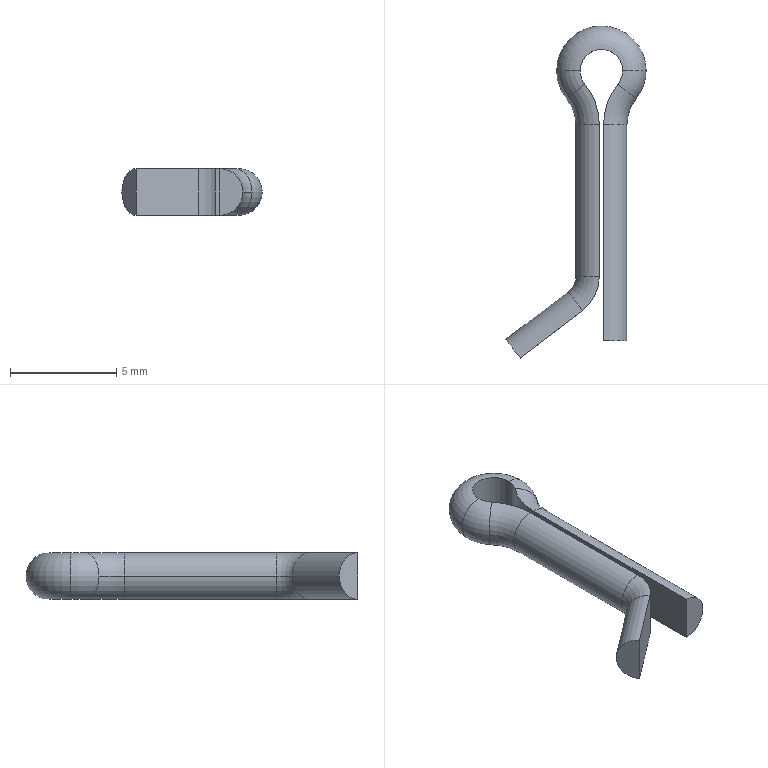Part | NX | features BREP 1 | 1 solid | 25 faces | box 6.586 x 15.587 x 2.2 mm | volume 61.721 mm3 | cylinder 11 | torus 9 | plane 5 | commonest cylinder face diameters 2.2 x5 2 x3 6 x2 4 x1
STEP:
#1=CARTESIAN_POINT('',(1.2,-6.604,4.));
#2=VERTEX_POINT('',#1);
#3=CARTESIAN_POINT('',(1.2,3.554,4.));
#4=VERTEX_POINT('',#3);
#5=CARTESIAN_POINT('',(1.2,-6.604,4.));
#6=DIRECTION('',(0.,1.,0.));
#7=VECTOR('',#6,1000.);
#8=LINE('',#5,#7);
#9=EDGE_CURVE('',#2,#4,#8,.T.);
#10=ORIENTED_EDGE('',*,*,#9,.F.);
#11=CARTESIAN_POINT('',(0.1,-6.604,2.9));
#12=VERTEX_POINT('',#11);
#13=CARTESIAN_POINT('',(0.1,-6.604,4.));
#14=DIRECTION('',(0.,-1.,0.));
#15=DIRECTION('',(0.,0.,-1.));
#16=AXIS2_PLACEMENT_3D('',#13,#14,#15);
#17=CIRCLE('',#16,1.1);
#18=EDGE_CURVE('',#12,#2,#17,.T.);
#19=ORIENTED_EDGE('',*,*,#18,.F.);
#20=CARTESIAN_POINT('',(0.1,3.554,2.9));
#21=VERTEX_POINT('',#20);
#22=CARTESIAN_POINT('',(0.1,-6.604,2.9));
#23=DIRECTION('',(0.,1.,0.));
#24=VECTOR('',#23,1000.);
#25=LINE('',#22,#24);
#26=EDGE_CURVE('',#12,#21,#25,.T.);
#27=ORIENTED_EDGE('',*,*,#26,.T.);
#28=CARTESIAN_POINT('',(0.1,3.554,4.));
#29=DIRECTION('',(0.,1.,0.));
#30=DIRECTION('',(1.,0.,0.));
#31=AXIS2_PLACEMENT_3D('',#28,#29,#30);
#32=CIRCLE('',#31,1.1);
#33=EDGE_CURVE('',#4,#21,#32,.T.);
#34=ORIENTED_EDGE('',*,*,#33,.F.);
#35=EDGE_LOOP('',(#10,#19,#27,#34));
#36=FACE_BOUND('',#35,.T.);
#37=CARTESIAN_POINT('',(0.1,3.554,4.));
#38=DIRECTION('',(0.,-1.,0.));
#39=DIRECTION('',(-1.,0.,0.));
#40=AXIS2_PLACEMENT_3D('',#37,#38,#39);
#41=CYLINDRICAL_SURFACE('',#40,1.1);
#42=ADVANCED_FACE('',(#36),#41,.T.);
#43=CARTESIAN_POINT('',(1.627,4.754,4.));
#44=VERTEX_POINT('',#43);
#45=CARTESIAN_POINT('',(3.1,3.554,4.));
#46=DIRECTION('',(0.,0.,-1.));
#47=DIRECTION('',(-1.,0.,0.));
#48=AXIS2_PLACEMENT_3D('',#45,#46,#47);
#49=CIRCLE('',#48,1.9);
#50=EDGE_CURVE('',#4,#44,#49,.T.);
#51=ORIENTED_EDGE('',*,*,#50,.F.);
#52=ORIENTED_EDGE('',*,*,#33,.T.);
#53=CARTESIAN_POINT('',(0.775,5.449,2.9));
#54=VERTEX_POINT('',#53);
#55=CARTESIAN_POINT('',(3.1,3.554,2.9));
#56=DIRECTION('',(0.,0.,-1.));
#57=DIRECTION('',(-1.,0.,0.));
#58=AXIS2_PLACEMENT_3D('',#55,#56,#57);
#59=CIRCLE('',#58,3.);
#60=EDGE_CURVE('',#21,#54,#59,.T.);
#61=ORIENTED_EDGE('',*,*,#60,.T.);
#62=CARTESIAN_POINT('',(0.775,5.449,4.));
#63=DIRECTION('',(-0.632,-0.775,0.));
#64=DIRECTION('',(0.,0.,-1.));
#65=AXIS2_PLACEMENT_3D('',#62,#63,#64);
#66=CIRCLE('',#65,1.1);
#67=EDGE_CURVE('',#54,#44,#66,.T.);
#68=ORIENTED_EDGE('',*,*,#67,.T.);
#69=EDGE_LOOP('',(#51,#52,#61,#68));
#70=FACE_BOUND('',#69,.T.);
#71=CARTESIAN_POINT('',(3.1,3.554,4.));
#72=DIRECTION('',(0.,0.,1.));
#73=DIRECTION('',(-1.,0.,0.));
#74=AXIS2_PLACEMENT_3D('',#71,#72,#73);
#75=TOROIDAL_SURFACE('',#74,3.,1.1);
#76=ADVANCED_FACE('',(#70),#75,.T.);
#77=CARTESIAN_POINT('',(2.1,6.081,4.));
#78=VERTEX_POINT('',#77);
#79=CARTESIAN_POINT('',(1.,6.081,5.1));
#80=VERTEX_POINT('',#79);
#81=CARTESIAN_POINT('',(1.,6.081,4.));
#82=DIRECTION('',(0.,-1.,0.));
#83=DIRECTION('',(1.,0.,0.));
#84=AXIS2_PLACEMENT_3D('',#81,#82,#83);
#85=CIRCLE('',#84,1.1);
#86=EDGE_CURVE('',#78,#80,#85,.T.);
#87=ORIENTED_EDGE('',*,*,#86,.T.);
#88=CARTESIAN_POINT('',(0.775,5.449,5.1));
#89=VERTEX_POINT('',#88);
#90=CARTESIAN_POINT('',(0.,6.081,5.1));
#91=DIRECTION('',(0.,0.,-1.));
#92=DIRECTION('',(1.,0.,0.));
#93=AXIS2_PLACEMENT_3D('',#90,#91,#92);
#94=CIRCLE('',#93,1.);
#95=EDGE_CURVE('',#80,#89,#94,.T.);
#96=ORIENTED_EDGE('',*,*,#95,.T.);
#97=CARTESIAN_POINT('',(0.775,5.449,4.));
#98=DIRECTION('',(-0.632,-0.775,0.));
#99=DIRECTION('',(0.775,-0.632,0.));
#100=AXIS2_PLACEMENT_3D('',#97,#98,#99);
#101=CIRCLE('',#100,1.1);
#102=EDGE_CURVE('',#44,#89,#101,.T.);
#103=ORIENTED_EDGE('',*,*,#102,.F.);
#104=ORIENTED_EDGE('',*,*,#67,.F.);
#105=CARTESIAN_POINT('',(1.,6.081,2.9));
#106=VERTEX_POINT('',#105);
#107=CARTESIAN_POINT('',(0.,6.081,2.9));
#108=DIRECTION('',(0.,0.,1.));
#109=DIRECTION('',(0.775,-0.632,0.));
#110=AXIS2_PLACEMENT_3D('',#107,#108,#109);
#111=CIRCLE('',#110,1.);
#112=EDGE_CURVE('',#54,#106,#111,.T.);
#113=ORIENTED_EDGE('',*,*,#112,.T.);
#114=CARTESIAN_POINT('',(1.,6.081,4.));
#115=DIRECTION('',(0.,-1.,0.));
#116=DIRECTION('',(0.,0.,-1.));
#117=AXIS2_PLACEMENT_3D('',#114,#115,#116);
#118=CIRCLE('',#117,1.1);
#119=EDGE_CURVE('',#106,#78,#118,.T.);
#120=ORIENTED_EDGE('',*,*,#119,.T.);
#121=EDGE_LOOP('',(#87,#96,#103,#104,#113,#120));
#122=FACE_BOUND('',#121,.T.);
#123=CARTESIAN_POINT('',(0.,6.081,4.));
#124=DIRECTION('',(0.,0.,-1.));
#125=DIRECTION('',(-1.,0.,0.));
#126=AXIS2_PLACEMENT_3D('',#123,#124,#125);
#127=DEGENERATE_TOROIDAL_SURFACE('',#126,1.,1.1,.T.);
#128=ADVANCED_FACE('',(#122),#127,.T.);
#129=ORIENTED_EDGE('',*,*,#86,.F.);
#130=ORIENTED_EDGE('',*,*,#119,.F.);
#131=CARTESIAN_POINT('',(-1.,6.081,2.9));
#132=VERTEX_POINT('',#131);
#133=CARTESIAN_POINT('',(0.,6.081,2.9));
#134=DIRECTION('',(0.,0.,1.));
#135=DIRECTION('',(1.,0.,0.));
#136=AXIS2_PLACEMENT_3D('',#133,#134,#135);
#137=CIRCLE('',#136,1.);
#138=EDGE_CURVE('',#106,#132,#137,.T.);
#139=ORIENTED_EDGE('',*,*,#138,.T.);
#140=CARTESIAN_POINT('',(-2.1,6.081,4.));
#141=VERTEX_POINT('',#140);
#142=CARTESIAN_POINT('',(-1.,6.081,4.));
#143=DIRECTION('',(0.,1.,0.));
#144=DIRECTION('',(0.,0.,-1.));
#145=AXIS2_PLACEMENT_3D('',#142,#143,#144);
#146=CIRCLE('',#145,1.1);
#147=EDGE_CURVE('',#132,#141,#146,.T.);
#148=ORIENTED_EDGE('',*,*,#147,.T.);
#149=CARTESIAN_POINT('',(-1.,6.081,5.1));
#150=VERTEX_POINT('',#149);
#151=CARTESIAN_POINT('',(-1.,6.081,4.));
#152=DIRECTION('',(0.,1.,0.));
#153=DIRECTION('',(-1.,0.,0.));
#154=AXIS2_PLACEMENT_3D('',#151,#152,#153);
#155=CIRCLE('',#154,1.1);
#156=EDGE_CURVE('',#141,#150,#155,.T.);
#157=ORIENTED_EDGE('',*,*,#156,.T.);
#158=CARTESIAN_POINT('',(0.,6.081,5.1));
#159=DIRECTION('',(0.,0.,-1.));
#160=DIRECTION('',(-1.,0.,0.));
#161=AXIS2_PLACEMENT_3D('',#158,#159,#160);
#162=CIRCLE('',#161,1.);
#163=EDGE_CURVE('',#150,#80,#162,.T.);
#164=ORIENTED_EDGE('',*,*,#163,.T.);
#165=EDGE_LOOP('',(#129,#130,#139,#148,#157,#164));
#166=FACE_BOUND('',#165,.T.);
#167=CARTESIAN_POINT('',(0.,6.081,4.));
#168=DIRECTION('',(0.,0.,-1.));
#169=DIRECTION('',(-1.,0.,0.));
#170=AXIS2_PLACEMENT_3D('',#167,#168,#169);
#171=DEGENERATE_TOROIDAL_SURFACE('',#170,1.,1.1,.T.);
#172=ADVANCED_FACE('',(#166),#171,.T.);
#173=ORIENTED_EDGE('',*,*,#163,.F.);
#174=CARTESIAN_POINT('',(-1.,6.081,2.9));
#175=DIRECTION('',(0.,0.,1.));
#176=VECTOR('',#175,1000.);
#177=LINE('',#174,#176);
#178=EDGE_CURVE('',#132,#150,#177,.T.);
#179=ORIENTED_EDGE('',*,*,#178,.F.);
#180=ORIENTED_EDGE('',*,*,#138,.F.);
#181=CARTESIAN_POINT('',(1.,6.081,2.9));
#182=DIRECTION('',(0.,0.,1.));
#183=VECTOR('',#182,1000.);
#184=LINE('',#181,#183);
#185=EDGE_CURVE('',#106,#80,#184,.T.);
#186=ORIENTED_EDGE('',*,*,#185,.T.);
#187=EDGE_LOOP('',(#173,#179,#180,#186));
#188=FACE_BOUND('',#187,.T.);
#189=CARTESIAN_POINT('',(0.,6.081,4.));
#190=DIRECTION('',(0.,0.,-1.));
#191=DIRECTION('',(1.,0.,0.));
#192=AXIS2_PLACEMENT_3D('',#189,#190,#191);
#193=CYLINDRICAL_SURFACE('',#192,1.);
#194=ADVANCED_FACE('',(#188),#193,.F.);
#195=ORIENTED_EDGE('',*,*,#185,.F.);
#196=ORIENTED_EDGE('',*,*,#112,.F.);
#197=CARTESIAN_POINT('',(0.775,5.449,5.1));
#198=DIRECTION('',(0.,0.,-1.));
#199=VECTOR('',#198,1000.);
#200=LINE('',#197,#199);
#201=EDGE_CURVE('',#89,#54,#200,.T.);
#202=ORIENTED_EDGE('',*,*,#201,.F.);
#203=ORIENTED_EDGE('',*,*,#95,.F.);
#204=EDGE_LOOP('',(#195,#196,#202,#203));
#205=FACE_BOUND('',#204,.T.);
#206=CARTESIAN_POINT('',(0.,6.081,4.));
#207=DIRECTION('',(0.,0.,-1.));
#208=DIRECTION('',(1.,0.,0.));
#209=AXIS2_PLACEMENT_3D('',#206,#207,#208);
#210=CYLINDRICAL_SURFACE('',#209,1.);
#211=ADVANCED_FACE('',(#205),#210,.F.);
#212=ORIENTED_EDGE('',*,*,#60,.F.);
#213=CARTESIAN_POINT('',(0.1,3.554,5.1));
#214=VERTEX_POINT('',#213);
#215=CARTESIAN_POINT('',(0.1,3.554,2.9));
#216=DIRECTION('',(0.,0.,1.));
#217=VECTOR('',#216,1000.);
#218=LINE('',#215,#217);
#219=EDGE_CURVE('',#21,#214,#218,.T.);
#220=ORIENTED_EDGE('',*,*,#219,.T.);
#221=CARTESIAN_POINT('',(3.1,3.554,5.1));
#222=DIRECTION('',(0.,0.,1.));
#223=DIRECTION('',(-0.775,0.632,0.));
#224=AXIS2_PLACEMENT_3D('',#221,#222,#223);
#225=CIRCLE('',#224,3.);
#226=EDGE_CURVE('',#89,#214,#225,.T.);
#227=ORIENTED_EDGE('',*,*,#226,.F.);
#228=ORIENTED_EDGE('',*,*,#201,.T.);
#229=EDGE_LOOP('',(#212,#220,#227,#228));
#230=FACE_BOUND('',#229,.T.);
#231=CARTESIAN_POINT('',(3.1,3.554,4.));
#232=DIRECTION('',(0.,0.,1.));
#233=DIRECTION('',(-1.,0.,0.));
#234=AXIS2_PLACEMENT_3D('',#231,#232,#233);
#235=CYLINDRICAL_SURFACE('',#234,3.);
#236=ADVANCED_FACE('',(#230),#235,.T.);
#237=ORIENTED_EDGE('',*,*,#102,.T.);
#238=ORIENTED_EDGE('',*,*,#226,.T.);
#239=CARTESIAN_POINT('',(0.1,3.554,4.));
#240=DIRECTION('',(0.,1.,0.));
#241=DIRECTION('',(0.,0.,1.));
#242=AXIS2_PLACEMENT_3D('',#239,#240,#241);
#243=CIRCLE('',#242,1.1);
#244=EDGE_CURVE('',#214,#4,#243,.T.);
#245=ORIENTED_EDGE('',*,*,#244,.T.);
#246=ORIENTED_EDGE('',*,*,#50,.T.);
#247=EDGE_LOOP('',(#237,#238,#245,#246));
#248=FACE_BOUND('',#247,.T.);
#249=CARTESIAN_POINT('',(3.1,3.554,4.));
#250=DIRECTION('',(0.,0.,1.));
#251=DIRECTION('',(-1.,0.,0.));
#252=AXIS2_PLACEMENT_3D('',#249,#250,#251);
#253=TOROIDAL_SURFACE('',#252,3.,1.1);
#254=ADVANCED_FACE('',(#248),#253,.T.);
#255=ORIENTED_EDGE('',*,*,#244,.F.);
#256=CARTESIAN_POINT('',(0.1,-6.604,5.1));
#257=VERTEX_POINT('',#256);
#258=CARTESIAN_POINT('',(0.1,3.554,5.1));
#259=DIRECTION('',(0.,-1.,0.));
#260=VECTOR('',#259,1000.);
#261=LINE('',#258,#260);
#262=EDGE_CURVE('',#214,#257,#261,.T.);
#263=ORIENTED_EDGE('',*,*,#262,.T.);
#264=CARTESIAN_POINT('',(0.1,-6.604,4.));
#265=DIRECTION('',(0.,-1.,0.));
#266=DIRECTION('',(1.,0.,0.));
#267=AXIS2_PLACEMENT_3D('',#264,#265,#266);
#268=CIRCLE('',#267,1.1);
#269=EDGE_CURVE('',#2,#257,#268,.T.);
#270=ORIENTED_EDGE('',*,*,#269,.F.);
#271=ORIENTED_EDGE('',*,*,#9,.T.);
#272=EDGE_LOOP('',(#255,#263,#270,#271));
#273=FACE_BOUND('',#272,.T.);
#274=CARTESIAN_POINT('',(0.1,3.554,4.));
#275=DIRECTION('',(0.,-1.,0.));
#276=DIRECTION('',(-1.,0.,0.));
#277=AXIS2_PLACEMENT_3D('',#274,#275,#276);
#278=CYLINDRICAL_SURFACE('',#277,1.1);
#279=ADVANCED_FACE('',(#273),#278,.T.);
#280=CARTESIAN_POINT('',(0.1,-6.604,5.1));
#281=DIRECTION('',(0.,0.,-1.));
#282=VECTOR('',#281,1000.);
#283=LINE('',#280,#282);
#284=EDGE_CURVE('',#257,#12,#283,.T.);
#285=ORIENTED_EDGE('',*,*,#284,.T.);
#286=ORIENTED_EDGE('',*,*,#18,.T.);
#287=ORIENTED_EDGE('',*,*,#269,.T.);
#288=EDGE_LOOP('',(#285,#286,#287));
#289=FACE_BOUND('',#288,.T.);
#290=CARTESIAN_POINT('',(0.1,-6.604,4.));
#291=DIRECTION('',(0.,1.,0.));
#292=DIRECTION('',(1.,0.,0.));
#293=AXIS2_PLACEMENT_3D('',#290,#291,#292);
#294=PLANE('',#293);
#295=ADVANCED_FACE('',(#289),#294,.F.);
#296=ORIENTED_EDGE('',*,*,#26,.F.);
#297=ORIENTED_EDGE('',*,*,#284,.F.);
#298=ORIENTED_EDGE('',*,*,#262,.F.);
#299=ORIENTED_EDGE('',*,*,#219,.F.);
#300=EDGE_LOOP('',(#296,#297,#298,#299));
#301=FACE_BOUND('',#300,.T.);
#302=CARTESIAN_POINT('',(0.1,3.554,5.1));
#303=DIRECTION('',(1.,0.,0.));
#304=DIRECTION('',(0.,-1.,0.));
#305=AXIS2_PLACEMENT_3D('',#302,#303,#304);
#306=PLANE('',#305);
#307=ADVANCED_FACE('',(#301),#306,.F.);
#308=CARTESIAN_POINT('',(-0.775,5.449,5.1));
#309=VERTEX_POINT('',#308);
#310=CARTESIAN_POINT('',(0.,6.081,5.1));
#311=DIRECTION('',(0.,0.,-1.));
#312=DIRECTION('',(-0.775,-0.632,0.));
#313=AXIS2_PLACEMENT_3D('',#310,#311,#312);
#314=CIRCLE('',#313,1.);
#315=EDGE_CURVE('',#309,#150,#314,.T.);
#316=ORIENTED_EDGE('',*,*,#315,.F.);
#317=CARTESIAN_POINT('',(-0.775,5.449,2.9));
#318=VERTEX_POINT('',#317);
#319=CARTESIAN_POINT('',(-0.775,5.449,5.1));
#320=DIRECTION('',(0.,0.,-1.));
#321=VECTOR('',#320,1000.);
#322=LINE('',#319,#321);
#323=EDGE_CURVE('',#309,#318,#322,.T.);
#324=ORIENTED_EDGE('',*,*,#323,.T.);
#325=CARTESIAN_POINT('',(0.,6.081,2.9));
#326=DIRECTION('',(0.,0.,1.));
#327=DIRECTION('',(-1.,0.,0.));
#328=AXIS2_PLACEMENT_3D('',#325,#326,#327);
#329=CIRCLE('',#328,1.);
#330=EDGE_CURVE('',#132,#318,#329,.T.);
#331=ORIENTED_EDGE('',*,*,#330,.F.);
#332=ORIENTED_EDGE('',*,*,#178,.T.);
#333=EDGE_LOOP('',(#316,#324,#331,#332));
#334=FACE_BOUND('',#333,.T.);
#335=CARTESIAN_POINT('',(0.,6.081,4.));
#336=DIRECTION('',(0.,0.,-1.));
#337=DIRECTION('',(1.,0.,0.));
#338=AXIS2_PLACEMENT_3D('',#335,#336,#337);
#339=CYLINDRICAL_SURFACE('',#338,1.);
#340=ADVANCED_FACE('',(#334),#339,.F.);
#341=ORIENTED_EDGE('',*,*,#156,.F.);
#342=ORIENTED_EDGE('',*,*,#147,.F.);
#343=ORIENTED_EDGE('',*,*,#330,.T.);
#344=CARTESIAN_POINT('',(-1.627,4.754,4.));
#345=VERTEX_POINT('',#344);
#346=CARTESIAN_POINT('',(-0.775,5.449,4.));
#347=DIRECTION('',(-0.632,0.775,0.));
#348=DIRECTION('',(0.,0.,-1.));
#349=AXIS2_PLACEMENT_3D('',#346,#347,#348);
#350=CIRCLE('',#349,1.1);
#351=EDGE_CURVE('',#318,#345,#350,.T.);
#352=ORIENTED_EDGE('',*,*,#351,.T.);
#353=CARTESIAN_POINT('',(-0.775,5.449,4.));
#354=DIRECTION('',(-0.632,0.775,0.));
#355=DIRECTION('',(-0.775,-0.632,0.));
#356=AXIS2_PLACEMENT_3D('',#353,#354,#355);
#357=CIRCLE('',#356,1.1);
#358=EDGE_CURVE('',#345,#309,#357,.T.);
#359=ORIENTED_EDGE('',*,*,#358,.T.);
#360=ORIENTED_EDGE('',*,*,#315,.T.);
#361=EDGE_LOOP('',(#341,#342,#343,#352,#359,#360));
#362=FACE_BOUND('',#361,.T.);
#363=CARTESIAN_POINT('',(0.,6.081,4.));
#364=DIRECTION('',(0.,0.,-1.));
#365=DIRECTION('',(-1.,0.,0.));
#366=AXIS2_PLACEMENT_3D('',#363,#364,#365);
#367=DEGENERATE_TOROIDAL_SURFACE('',#366,1.,1.1,.T.);
#368=ADVANCED_FACE('',(#362),#367,.T.);
#369=CARTESIAN_POINT('',(-1.2,3.554,4.));
#370=VERTEX_POINT('',#369);
#371=CARTESIAN_POINT('',(-0.1,3.554,5.1));
#372=VERTEX_POINT('',#371);
#373=CARTESIAN_POINT('',(-0.1,3.554,4.));
#374=DIRECTION('',(0.,1.,0.));
#375=DIRECTION('',(-1.,0.,0.));
#376=AXIS2_PLACEMENT_3D('',#373,#374,#375);
#377=CIRCLE('',#376,1.1);
#378=EDGE_CURVE('',#370,#372,#377,.T.);
#379=ORIENTED_EDGE('',*,*,#378,.T.);
#380=CARTESIAN_POINT('',(-3.1,3.554,5.1));
#381=DIRECTION('',(0.,0.,1.));
#382=DIRECTION('',(1.,0.,0.));
#383=AXIS2_PLACEMENT_3D('',#380,#381,#382);
#384=CIRCLE('',#383,3.);
#385=EDGE_CURVE('',#372,#309,#384,.T.);
#386=ORIENTED_EDGE('',*,*,#385,.T.);
#387=ORIENTED_EDGE('',*,*,#358,.F.);
#388=CARTESIAN_POINT('',(-3.1,3.554,4.));
#389=DIRECTION('',(0.,0.,-1.));
#390=DIRECTION('',(0.775,0.632,0.));
#391=AXIS2_PLACEMENT_3D('',#388,#389,#390);
#392=CIRCLE('',#391,1.9);
#393=EDGE_CURVE('',#345,#370,#392,.T.);
#394=ORIENTED_EDGE('',*,*,#393,.T.);
#395=EDGE_LOOP('',(#379,#386,#387,#394));
#396=FACE_BOUND('',#395,.T.);
#397=CARTESIAN_POINT('',(-3.1,3.554,4.));
#398=DIRECTION('',(0.,0.,1.));
#399=DIRECTION('',(-1.,0.,0.));
#400=AXIS2_PLACEMENT_3D('',#397,#398,#399);
#401=TOROIDAL_SURFACE('',#400,3.,1.1);
#402=ADVANCED_FACE('',(#396),#401,.T.);
#403=ORIENTED_EDGE('',*,*,#393,.F.);
#404=ORIENTED_EDGE('',*,*,#351,.F.);
#405=CARTESIAN_POINT('',(-0.1,3.554,2.9));
#406=VERTEX_POINT('',#405);
#407=CARTESIAN_POINT('',(-3.1,3.554,2.9));
#408=DIRECTION('',(0.,0.,-1.));
#409=DIRECTION('',(0.775,0.632,0.));
#410=AXIS2_PLACEMENT_3D('',#407,#408,#409);
#411=CIRCLE('',#410,3.);
#412=EDGE_CURVE('',#318,#406,#411,.T.);
#413=ORIENTED_EDGE('',*,*,#412,.T.);
#414=CARTESIAN_POINT('',(-0.1,3.554,4.));
#415=DIRECTION('',(0.,1.,0.));
#416=DIRECTION('',(0.,0.,-1.));
#417=AXIS2_PLACEMENT_3D('',#414,#415,#416);
#418=CIRCLE('',#417,1.1);
#419=EDGE_CURVE('',#406,#370,#418,.T.);
#420=ORIENTED_EDGE('',*,*,#419,.T.);
#421=EDGE_LOOP('',(#403,#404,#413,#420));
#422=FACE_BOUND('',#421,.T.);
#423=CARTESIAN_POINT('',(-3.1,3.554,4.));
#424=DIRECTION('',(0.,0.,1.));
#425=DIRECTION('',(-1.,0.,0.));
#426=AXIS2_PLACEMENT_3D('',#423,#424,#425);
#427=TOROIDAL_SURFACE('',#426,3.,1.1);
#428=ADVANCED_FACE('',(#422),#427,.T.);
#429=CARTESIAN_POINT('',(-1.2,-3.591,4.));
#430=VERTEX_POINT('',#429);
#431=CARTESIAN_POINT('',(-1.2,3.554,4.));
#432=DIRECTION('',(0.,-1.,0.));
#433=VECTOR('',#432,1000.);
#434=LINE('',#431,#433);
#435=EDGE_CURVE('',#370,#430,#434,.T.);
#436=ORIENTED_EDGE('',*,*,#435,.F.);
#437=ORIENTED_EDGE('',*,*,#419,.F.);
#438=CARTESIAN_POINT('',(-0.1,-3.591,2.9));
#439=VERTEX_POINT('',#438);
#440=CARTESIAN_POINT('',(-0.1,3.554,2.9));
#441=DIRECTION('',(0.,-1.,0.));
#442=VECTOR('',#441,1000.);
#443=LINE('',#440,#442);
#444=EDGE_CURVE('',#406,#439,#443,.T.);
#445=ORIENTED_EDGE('',*,*,#444,.T.);
#446=CARTESIAN_POINT('',(-0.1,-3.591,4.));
#447=DIRECTION('',(0.,-1.,0.));
#448=DIRECTION('',(-1.,0.,0.));
#449=AXIS2_PLACEMENT_3D('',#446,#447,#448);
#450=CIRCLE('',#449,1.1);
#451=EDGE_CURVE('',#430,#439,#450,.T.);
#452=ORIENTED_EDGE('',*,*,#451,.F.);
#453=EDGE_LOOP('',(#436,#437,#445,#452));
#454=FACE_BOUND('',#453,.T.);
#455=CARTESIAN_POINT('',(-0.1,-3.591,4.));
#456=DIRECTION('',(0.,1.,0.));
#457=DIRECTION('',(1.,0.,0.));
#458=AXIS2_PLACEMENT_3D('',#455,#456,#457);
#459=CYLINDRICAL_SURFACE('',#458,1.1);
#460=ADVANCED_FACE('',(#454),#459,.T.);
#461=CARTESIAN_POINT('',(-1.556,-4.308,4.));
#462=VERTEX_POINT('',#461);
#463=CARTESIAN_POINT('',(-2.1,-3.591,4.));
#464=DIRECTION('',(0.,0.,-1.));
#465=DIRECTION('',(1.,0.,0.));
#466=AXIS2_PLACEMENT_3D('',#463,#464,#465);
#467=CIRCLE('',#466,0.9);
#468=EDGE_CURVE('',#430,#462,#467,.T.);
#469=ORIENTED_EDGE('',*,*,#468,.F.);
#470=ORIENTED_EDGE('',*,*,#451,.T.);
#471=CARTESIAN_POINT('',(-0.8919,-5.185,2.9));
#472=VERTEX_POINT('',#471);
#473=CARTESIAN_POINT('',(-2.1,-3.591,2.9));
#474=DIRECTION('',(0.,0.,-1.));
#475=DIRECTION('',(1.,0.,0.));
#476=AXIS2_PLACEMENT_3D('',#473,#474,#475);
#477=CIRCLE('',#476,2.);
#478=EDGE_CURVE('',#439,#472,#477,.T.);
#479=ORIENTED_EDGE('',*,*,#478,.T.);
#480=CARTESIAN_POINT('',(-0.8919,-5.185,4.));
#481=DIRECTION('',(0.7969,0.6041,0.));
#482=DIRECTION('',(0.,0.,-1.));
#483=AXIS2_PLACEMENT_3D('',#480,#481,#482);
#484=CIRCLE('',#483,1.1);
#485=EDGE_CURVE('',#472,#462,#484,.T.);
#486=ORIENTED_EDGE('',*,*,#485,.T.);
#487=EDGE_LOOP('',(#469,#470,#479,#486));
#488=FACE_BOUND('',#487,.T.);
#489=CARTESIAN_POINT('',(-2.1,-3.591,4.));
#490=DIRECTION('',(0.,0.,1.));
#491=DIRECTION('',(-1.,0.,0.));
#492=AXIS2_PLACEMENT_3D('',#489,#490,#491);
#493=TOROIDAL_SURFACE('',#492,2.,1.1);
#494=ADVANCED_FACE('',(#488),#493,.T.);
#495=CARTESIAN_POINT('',(-3.822,-7.406,5.1));
#496=VERTEX_POINT('',#495);
#497=CARTESIAN_POINT('',(-4.486,-6.529,4.));
#498=VERTEX_POINT('',#497);
#499=CARTESIAN_POINT('',(-3.822,-7.406,4.));
#500=DIRECTION('',(-0.7969,-0.6041,0.));
#501=DIRECTION('',(0.,0.,1.));
#502=AXIS2_PLACEMENT_3D('',#499,#500,#501);
#503=CIRCLE('',#502,1.1);
#504=EDGE_CURVE('',#496,#498,#503,.T.);
#505=ORIENTED_EDGE('',*,*,#504,.F.);
#506=CARTESIAN_POINT('',(-0.8919,-5.185,5.1));
#507=VERTEX_POINT('',#506);
#508=CARTESIAN_POINT('',(-3.822,-7.406,5.1));
#509=DIRECTION('',(0.7969,0.6041,0.));
#510=VECTOR('',#509,1000.);
#511=LINE('',#508,#510);
#512=EDGE_CURVE('',#496,#507,#511,.T.);
#513=ORIENTED_EDGE('',*,*,#512,.T.);
#514=CARTESIAN_POINT('',(-0.8919,-5.185,4.));
#515=DIRECTION('',(0.7969,0.6041,0.));
#516=DIRECTION('',(-0.6041,0.7969,0.));
#517=AXIS2_PLACEMENT_3D('',#514,#515,#516);
#518=CIRCLE('',#517,1.1);
#519=EDGE_CURVE('',#462,#507,#518,.T.);
#520=ORIENTED_EDGE('',*,*,#519,.F.);
#521=ORIENTED_EDGE('',*,*,#485,.F.);
#522=CARTESIAN_POINT('',(-3.822,-7.406,2.9));
#523=VERTEX_POINT('',#522);
#524=CARTESIAN_POINT('',(-0.8919,-5.185,2.9));
#525=DIRECTION('',(-0.7969,-0.6041,0.));
#526=VECTOR('',#525,1000.);
#527=LINE('',#524,#526);
#528=EDGE_CURVE('',#472,#523,#527,.T.);
#529=ORIENTED_EDGE('',*,*,#528,.T.);
#530=CARTESIAN_POINT('',(-3.822,-7.406,4.));
#531=DIRECTION('',(-0.7969,-0.6041,0.));
#532=DIRECTION('',(-0.6041,0.7969,0.));
#533=AXIS2_PLACEMENT_3D('',#530,#531,#532);
#534=CIRCLE('',#533,1.1);
#535=EDGE_CURVE('',#498,#523,#534,.T.);
#536=ORIENTED_EDGE('',*,*,#535,.F.);
#537=EDGE_LOOP('',(#505,#513,#520,#521,#529,#536));
#538=FACE_BOUND('',#537,.T.);
#539=CARTESIAN_POINT('',(-0.8919,-5.185,4.));
#540=DIRECTION('',(-0.7969,-0.6041,0.));
#541=DIRECTION('',(-0.6041,0.7969,0.));
#542=AXIS2_PLACEMENT_3D('',#539,#540,#541);
#543=CYLINDRICAL_SURFACE('',#542,1.1);
#544=ADVANCED_FACE('',(#538),#543,.T.);
#545=ORIENTED_EDGE('',*,*,#535,.T.);
#546=CARTESIAN_POINT('',(-3.822,-7.406,5.1));
#547=DIRECTION('',(0.,0.,-1.));
#548=VECTOR('',#547,1000.);
#549=LINE('',#546,#548);
#550=EDGE_CURVE('',#496,#523,#549,.T.);
#551=ORIENTED_EDGE('',*,*,#550,.F.);
#552=ORIENTED_EDGE('',*,*,#504,.T.);
#553=EDGE_LOOP('',(#545,#551,#552));
#554=FACE_BOUND('',#553,.T.);
#555=CARTESIAN_POINT('',(-3.822,-7.406,4.));
#556=DIRECTION('',(-0.7969,-0.6041,0.));
#557=DIRECTION('',(-0.6041,0.7969,0.));
#558=AXIS2_PLACEMENT_3D('',#555,#556,#557);
#559=PLANE('',#558);
#560=ADVANCED_FACE('',(#554),#559,.T.);
#561=ORIENTED_EDGE('',*,*,#528,.F.);
#562=CARTESIAN_POINT('',(-0.8919,-5.185,5.1));
#563=DIRECTION('',(0.,0.,-1.));
#564=VECTOR('',#563,1000.);
#565=LINE('',#562,#564);
#566=EDGE_CURVE('',#507,#472,#565,.T.);
#567=ORIENTED_EDGE('',*,*,#566,.F.);
#568=ORIENTED_EDGE('',*,*,#512,.F.);
#569=ORIENTED_EDGE('',*,*,#550,.T.);
#570=EDGE_LOOP('',(#561,#567,#568,#569));
#571=FACE_BOUND('',#570,.T.);
#572=CARTESIAN_POINT('',(-0.8919,-5.185,5.1));
#573=DIRECTION('',(0.6041,-0.7969,0.));
#574=DIRECTION('',(-0.7969,-0.6041,0.));
#575=AXIS2_PLACEMENT_3D('',#572,#573,#574);
#576=PLANE('',#575);
#577=ADVANCED_FACE('',(#571),#576,.T.);
#578=ORIENTED_EDGE('',*,*,#478,.F.);
#579=CARTESIAN_POINT('',(-0.1,-3.591,5.1));
#580=VERTEX_POINT('',#579);
#581=CARTESIAN_POINT('',(-0.1,-3.591,2.9));
#582=DIRECTION('',(0.,0.,1.));
#583=VECTOR('',#582,1000.);
#584=LINE('',#581,#583);
#585=EDGE_CURVE('',#439,#580,#584,.T.);
#586=ORIENTED_EDGE('',*,*,#585,.T.);
#587=CARTESIAN_POINT('',(-2.1,-3.591,5.1));
#588=DIRECTION('',(0.,0.,1.));
#589=DIRECTION('',(0.6041,-0.7969,0.));
#590=AXIS2_PLACEMENT_3D('',#587,#588,#589);
#591=CIRCLE('',#590,2.);
#592=EDGE_CURVE('',#507,#580,#591,.T.);
#593=ORIENTED_EDGE('',*,*,#592,.F.);
#594=ORIENTED_EDGE('',*,*,#566,.T.);
#595=EDGE_LOOP('',(#578,#586,#593,#594));
#596=FACE_BOUND('',#595,.T.);
#597=CARTESIAN_POINT('',(-2.1,-3.591,4.));
#598=DIRECTION('',(0.,0.,1.));
#599=DIRECTION('',(-1.,0.,0.));
#600=AXIS2_PLACEMENT_3D('',#597,#598,#599);
#601=CYLINDRICAL_SURFACE('',#600,2.);
#602=ADVANCED_FACE('',(#596),#601,.T.);
#603=ORIENTED_EDGE('',*,*,#519,.T.);
#604=ORIENTED_EDGE('',*,*,#592,.T.);
#605=CARTESIAN_POINT('',(-0.1,-3.591,4.));
#606=DIRECTION('',(0.,-1.,0.));
#607=DIRECTION('',(0.,0.,1.));
#608=AXIS2_PLACEMENT_3D('',#605,#606,#607);
#609=CIRCLE('',#608,1.1);
#610=EDGE_CURVE('',#580,#430,#609,.T.);
#611=ORIENTED_EDGE('',*,*,#610,.T.);
#612=ORIENTED_EDGE('',*,*,#468,.T.);
#613=EDGE_LOOP('',(#603,#604,#611,#612));
#614=FACE_BOUND('',#613,.T.);
#615=CARTESIAN_POINT('',(-2.1,-3.591,4.));
#616=DIRECTION('',(0.,0.,1.));
#617=DIRECTION('',(-1.,0.,0.));
#618=AXIS2_PLACEMENT_3D('',#615,#616,#617);
#619=TOROIDAL_SURFACE('',#618,2.,1.1);
#620=ADVANCED_FACE('',(#614),#619,.T.);
#621=ORIENTED_EDGE('',*,*,#610,.F.);
#622=CARTESIAN_POINT('',(-0.1,-3.591,5.1));
#623=DIRECTION('',(0.,1.,0.));
#624=VECTOR('',#623,1000.);
#625=LINE('',#622,#624);
#626=EDGE_CURVE('',#580,#372,#625,.T.);
#627=ORIENTED_EDGE('',*,*,#626,.T.);
#628=ORIENTED_EDGE('',*,*,#378,.F.);
#629=ORIENTED_EDGE('',*,*,#435,.T.);
#630=EDGE_LOOP('',(#621,#627,#628,#629));
#631=FACE_BOUND('',#630,.T.);
#632=CARTESIAN_POINT('',(-0.1,-3.591,4.));
#633=DIRECTION('',(0.,1.,0.));
#634=DIRECTION('',(1.,0.,0.));
#635=AXIS2_PLACEMENT_3D('',#632,#633,#634);
#636=CYLINDRICAL_SURFACE('',#635,1.1);
#637=ADVANCED_FACE('',(#631),#636,.T.);
#638=ORIENTED_EDGE('',*,*,#444,.F.);
#639=CARTESIAN_POINT('',(-0.1,3.554,5.1));
#640=DIRECTION('',(0.,0.,-1.));
#641=VECTOR('',#640,1000.);
#642=LINE('',#639,#641);
#643=EDGE_CURVE('',#372,#406,#642,.T.);
#644=ORIENTED_EDGE('',*,*,#643,.F.);
#645=ORIENTED_EDGE('',*,*,#626,.F.);
#646=ORIENTED_EDGE('',*,*,#585,.F.);
#647=EDGE_LOOP('',(#638,#644,#645,#646));
#648=FACE_BOUND('',#647,.T.);
#649=CARTESIAN_POINT('',(-0.1,-3.591,5.1));
#650=DIRECTION('',(-1.,0.,0.));
#651=DIRECTION('',(0.,1.,0.));
#652=AXIS2_PLACEMENT_3D('',#649,#650,#651);
#653=PLANE('',#652);
#654=ADVANCED_FACE('',(#648),#653,.F.);
#655=ORIENTED_EDGE('',*,*,#412,.F.);
#656=ORIENTED_EDGE('',*,*,#323,.F.);
#657=ORIENTED_EDGE('',*,*,#385,.F.);
#658=ORIENTED_EDGE('',*,*,#643,.T.);
#659=EDGE_LOOP('',(#655,#656,#657,#658));
#660=FACE_BOUND('',#659,.T.);
#661=CARTESIAN_POINT('',(-3.1,3.554,4.));
#662=DIRECTION('',(0.,0.,1.));
#663=DIRECTION('',(-1.,0.,0.));
#664=AXIS2_PLACEMENT_3D('',#661,#662,#663);
#665=CYLINDRICAL_SURFACE('',#664,3.);
#666=ADVANCED_FACE('',(#660),#665,.T.);
#667=CLOSED_SHELL('',(#42,#76,#128,#172,#194,#211,#236,#254,#279,#295,#307,#340,#368,#402,#428,#460,#494,#544,#560,#577,#602,#620,#637,#654,#666));
#668=MANIFOLD_SOLID_BREP('',#667);
#669=(LENGTH_UNIT()NAMED_UNIT(*)SI_UNIT(.MILLI.,.METRE.));
#670=UNCERTAINTY_MEASURE_WITH_UNIT(LENGTH_MEASURE(0.00001),#669,'','');
#671=(NAMED_UNIT(*)PLANE_ANGLE_UNIT()SI_UNIT($,.RADIAN.));
#672=(NAMED_UNIT(*)SI_UNIT($,.STERADIAN.)SOLID_ANGLE_UNIT());
#673=(GEOMETRIC_REPRESENTATION_CONTEXT(3)GLOBAL_UNCERTAINTY_ASSIGNED_CONTEXT((#670))GLOBAL_UNIT_ASSIGNED_CONTEXT((#669,#671,#672))REPRESENTATION_CONTEXT('',''));
#674=ADVANCED_BREP_SHAPE_REPRESENTATION('',(#668),#673);